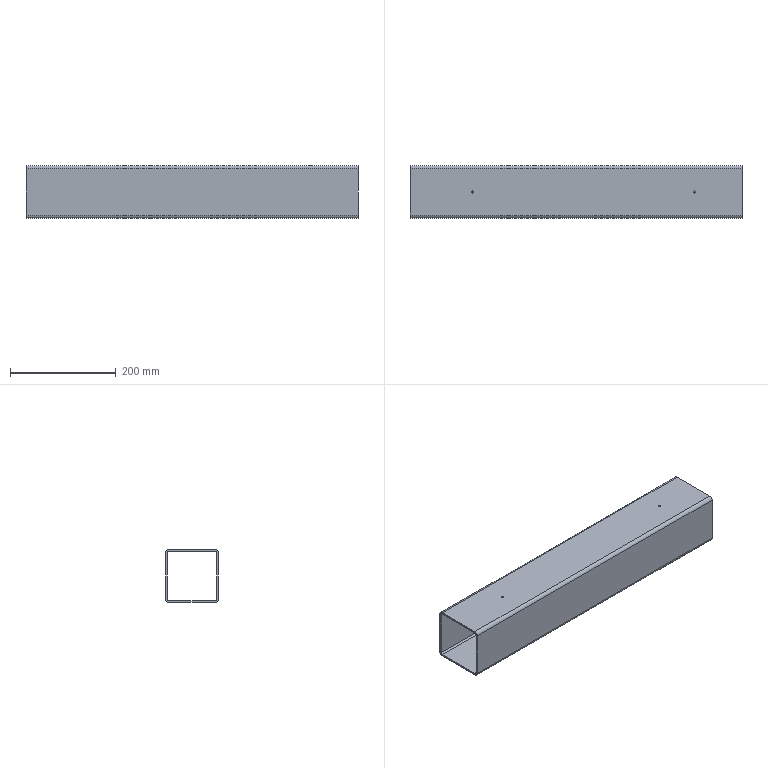Part | STEP file | [01]-1 | 1 solid | 22 faces | box 628 x 100 x 100 mm | volume 761476 mm3 | cylinder 12 | plane 10 | commonest cylinder face diameters 4 x4 6.4 x4 12.8 x4